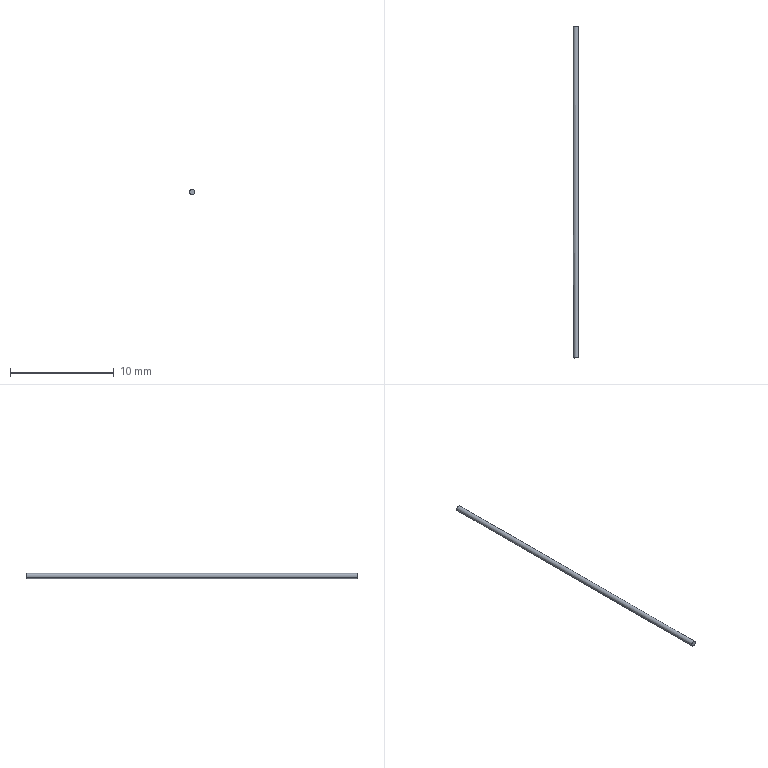Part | SolidWorks | features BaseBody 1 | 1 solid | 4 faces | box 0.5307 x 32 x 0.5 mm | volume 6.283 mm3 | cylinder 2 | plane 2 | commonest cylinder face diameters 0.5 x2
STEP:
#1=CARTESIAN_POINT('',(352.593,424.474,107.975));
#2=VERTEX_POINT('',#1);
#3=CARTESIAN_POINT('',(353.026,424.475,108.225));
#4=VERTEX_POINT('',#3);
#5=CARTESIAN_POINT('',(352.81,424.474,108.1));
#6=DIRECTION('',(-0.0009599,1.,0.));
#7=DIRECTION('',(0.866,0.0008313,0.5));
#8=AXIS2_PLACEMENT_3D('',#5,#6,#7);
#9=CIRCLE('',#8,0.25);
#10=EDGE_CURVE('',#2,#4,#9,.T.);
#11=ORIENTED_EDGE('',*,*,#10,.F.);
#12=CARTESIAN_POINT('',(352.624,392.474,107.975));
#13=VERTEX_POINT('',#12);
#14=CARTESIAN_POINT('',(352.593,424.474,107.975));
#15=DIRECTION('',(0.0009599,-1.,0.));
#16=VECTOR('',#15,1000.);
#17=LINE('',#14,#16);
#18=EDGE_CURVE('',#2,#13,#17,.T.);
#19=ORIENTED_EDGE('',*,*,#18,.T.);
#20=CARTESIAN_POINT('',(353.057,392.475,108.225));
#21=VERTEX_POINT('',#20);
#22=CARTESIAN_POINT('',(352.84,392.475,108.1));
#23=DIRECTION('',(0.0009599,-1.,0.));
#24=DIRECTION('',(0.866,0.0008313,0.5));
#25=AXIS2_PLACEMENT_3D('',#22,#23,#24);
#26=CIRCLE('',#25,0.25);
#27=EDGE_CURVE('',#21,#13,#26,.T.);
#28=ORIENTED_EDGE('',*,*,#27,.F.);
#29=CARTESIAN_POINT('',(353.026,424.475,108.225));
#30=DIRECTION('',(0.0009599,-1.,0.));
#31=VECTOR('',#30,1000.);
#32=LINE('',#29,#31);
#33=EDGE_CURVE('',#4,#21,#32,.T.);
#34=ORIENTED_EDGE('',*,*,#33,.F.);
#35=EDGE_LOOP('',(#11,#19,#28,#34));
#36=FACE_OUTER_BOUND('',#35,.T.);
#37=CARTESIAN_POINT('',(352.81,424.474,108.1));
#38=DIRECTION('',(0.0009599,-1.,0.));
#39=DIRECTION('',(0.866,0.0008313,0.5));
#40=AXIS2_PLACEMENT_3D('',#37,#38,#39);
#41=CYLINDRICAL_SURFACE('',#40,0.25);
#42=ADVANCED_FACE('',(#36),#41,.T.);
#43=CARTESIAN_POINT('',(352.81,424.474,108.1));
#44=DIRECTION('',(-0.0009599,1.,0.));
#45=DIRECTION('',(0.866,0.0008313,0.5));
#46=AXIS2_PLACEMENT_3D('',#43,#44,#45);
#47=CIRCLE('',#46,0.25);
#48=EDGE_CURVE('',#4,#2,#47,.T.);
#49=ORIENTED_EDGE('',*,*,#48,.T.);
#50=ORIENTED_EDGE('',*,*,#10,.T.);
#51=EDGE_LOOP('',(#49,#50));
#52=FACE_OUTER_BOUND('',#51,.T.);
#53=CARTESIAN_POINT('',(352.81,424.474,108.1));
#54=DIRECTION('',(-0.0009599,1.,0.));
#55=DIRECTION('',(0.,0.,1.));
#56=AXIS2_PLACEMENT_3D('',#53,#54,#55);
#57=PLANE('',#56);
#58=ADVANCED_FACE('',(#52),#57,.T.);
#59=ORIENTED_EDGE('',*,*,#18,.F.);
#60=ORIENTED_EDGE('',*,*,#48,.F.);
#61=ORIENTED_EDGE('',*,*,#33,.T.);
#62=CARTESIAN_POINT('',(352.84,392.475,108.1));
#63=DIRECTION('',(0.0009599,-1.,0.));
#64=DIRECTION('',(0.866,0.0008313,0.5));
#65=AXIS2_PLACEMENT_3D('',#62,#63,#64);
#66=CIRCLE('',#65,0.25);
#67=EDGE_CURVE('',#13,#21,#66,.T.);
#68=ORIENTED_EDGE('',*,*,#67,.F.);
#69=EDGE_LOOP('',(#59,#60,#61,#68));
#70=FACE_OUTER_BOUND('',#69,.T.);
#71=CARTESIAN_POINT('',(352.81,424.474,108.1));
#72=DIRECTION('',(0.0009599,-1.,0.));
#73=DIRECTION('',(0.866,0.0008313,0.5));
#74=AXIS2_PLACEMENT_3D('',#71,#72,#73);
#75=CYLINDRICAL_SURFACE('',#74,0.25);
#76=ADVANCED_FACE('',(#70),#75,.T.);
#77=ORIENTED_EDGE('',*,*,#27,.T.);
#78=ORIENTED_EDGE('',*,*,#67,.T.);
#79=EDGE_LOOP('',(#77,#78));
#80=FACE_OUTER_BOUND('',#79,.T.);
#81=CARTESIAN_POINT('',(352.84,392.475,108.1));
#82=DIRECTION('',(-0.0009599,1.,0.));
#83=DIRECTION('',(0.,0.,1.));
#84=AXIS2_PLACEMENT_3D('',#81,#82,#83);
#85=PLANE('',#84);
#86=ADVANCED_FACE('',(#80),#85,.F.);
#87=CLOSED_SHELL('',(#42,#58,#76,#86));
#88=MANIFOLD_SOLID_BREP('',#87);
#89=CARTESIAN_POINT('',(0.,0.,0.));
#90=DIRECTION('',(0.,0.,1.));
#91=DIRECTION('',(1.,0.,0.));
#92=AXIS2_PLACEMENT_3D('',#89,#90,#91);
#93=(LENGTH_UNIT()NAMED_UNIT(*)SI_UNIT(.MILLI.,.METRE.));
#94=UNCERTAINTY_MEASURE_WITH_UNIT(LENGTH_MEASURE(0.00001),#93,'','');
#95=(NAMED_UNIT(*)PLANE_ANGLE_UNIT()SI_UNIT($,.RADIAN.));
#96=(NAMED_UNIT(*)SI_UNIT($,.STERADIAN.)SOLID_ANGLE_UNIT());
#97=(GEOMETRIC_REPRESENTATION_CONTEXT(3)GLOBAL_UNCERTAINTY_ASSIGNED_CONTEXT((#94))GLOBAL_UNIT_ASSIGNED_CONTEXT((#93,#95,#96))REPRESENTATION_CONTEXT('',''));
#98=ADVANCED_BREP_SHAPE_REPRESENTATION('',(#88,#92),#97);